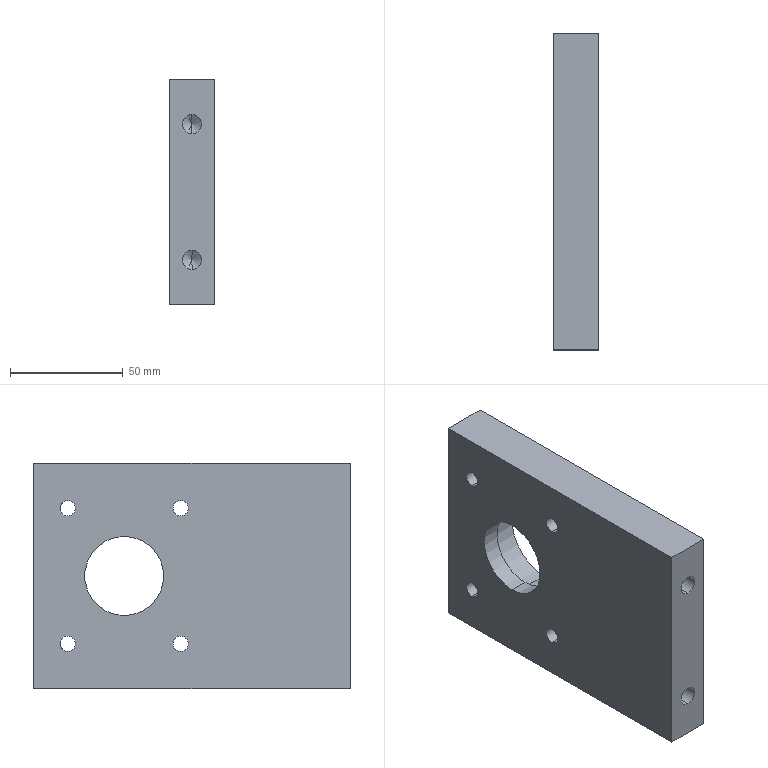Part | SolidWorks | features HoleWzd 3, ICE 2, Extrusion 1 | 1 solid | 31 faces | box 20 x 140 x 100 mm | volume 250976 mm3 | cylinder 20 | plane 7 | cone 4 | commonest cylinder face diameters 6.8 x8 5 x4 8.5 x4 35 x2 40 x2
STEP:
#1=CARTESIAN_POINT('',(10.,57.304,-32.5));
#2=VERTEX_POINT('',#1);
#3=CARTESIAN_POINT('',(10.,57.304,-27.5));
#4=VERTEX_POINT('',#3);
#5=CARTESIAN_POINT('',(10.,57.304,-32.5));
#6=CARTESIAN_POINT('',(9.828,57.304,-32.5));
#7=CARTESIAN_POINT('',(9.657,57.324,-32.482));
#8=CARTESIAN_POINT('',(9.329,57.395,-32.414));
#9=CARTESIAN_POINT('',(9.17,57.445,-32.364));
#10=CARTESIAN_POINT('',(8.728,57.618,-32.176));
#11=CARTESIAN_POINT('',(8.464,57.763,-31.998));
#12=CARTESIAN_POINT('',(8.13,57.966,-31.667));
#13=CARTESIAN_POINT('',(8.027,58.033,-31.544));
#14=CARTESIAN_POINT('',(7.847,58.153,-31.28));
#15=CARTESIAN_POINT('',(7.769,58.207,-31.139));
#16=CARTESIAN_POINT('',(7.638,58.299,-30.836));
#17=CARTESIAN_POINT('',(7.587,58.336,-30.675));
#18=CARTESIAN_POINT('',(7.519,58.386,-30.347));
#19=CARTESIAN_POINT('',(7.5,58.4,-30.176));
#20=CARTESIAN_POINT('',(7.5,58.4,-29.832));
#21=CARTESIAN_POINT('',(7.517,58.387,-29.663));
#22=CARTESIAN_POINT('',(7.585,58.338,-29.331));
#23=CARTESIAN_POINT('',(7.636,58.301,-29.169));
#24=CARTESIAN_POINT('',(7.766,58.209,-28.866));
#25=CARTESIAN_POINT('',(7.845,58.154,-28.722));
#26=CARTESIAN_POINT('',(8.026,58.033,-28.458));
#27=CARTESIAN_POINT('',(8.127,57.968,-28.336));
#28=CARTESIAN_POINT('',(8.464,57.764,-28.003));
#29=CARTESIAN_POINT('',(8.722,57.62,-27.827));
#30=CARTESIAN_POINT('',(9.17,57.445,-27.636));
#31=CARTESIAN_POINT('',(9.326,57.396,-27.587));
#32=CARTESIAN_POINT('',(9.655,57.325,-27.518));
#33=CARTESIAN_POINT('',(9.827,57.304,-27.5));
#34=CARTESIAN_POINT('',(10.,57.304,-27.5));
#35=B_SPLINE_CURVE_WITH_KNOTS('',3,(#5,#6,#7,#8,#9,#10,#11,#12,#13,#14,#15,#16,#17,#18,#19,#20,#21,#22,#23,#24,#25,#26,#27,#28,#29,#30,#31,#32,#33,#34),.UNSPECIFIED.,.F.,.F.,(4,2,2,2,2,2,2,2,2,2,2,2,2,2,4),(0.008147,0.008656,0.009164,0.01018,0.01069,0.0112,0.01171,0.01221,0.01272,0.01323,0.01374,0.01425,0.01526,0.01577,0.01628),.UNSPECIFIED.);
#36=EDGE_CURVE('',#2,#4,#35,.T.);
#37=ORIENTED_EDGE('',*,*,#36,.F.);
#38=CARTESIAN_POINT('',(10.,70.,-32.5));
#39=VERTEX_POINT('',#38);
#40=CARTESIAN_POINT('',(10.,70.,-32.5));
#41=DIRECTION('',(0.,1.,0.));
#42=VECTOR('',#41,1000.);
#43=LINE('',#40,#42);
#44=EDGE_CURVE('',#2,#39,#43,.T.);
#45=ORIENTED_EDGE('',*,*,#44,.T.);
#46=CARTESIAN_POINT('',(10.,70.,-27.5));
#47=VERTEX_POINT('',#46);
#48=CARTESIAN_POINT('',(10.,70.,-30.));
#49=DIRECTION('',(0.,1.,0.));
#50=DIRECTION('',(0.,0.,1.));
#51=AXIS2_PLACEMENT_3D('',#48,#49,#50);
#52=CIRCLE('',#51,2.5);
#53=EDGE_CURVE('',#39,#47,#52,.T.);
#54=ORIENTED_EDGE('',*,*,#53,.T.);
#55=CARTESIAN_POINT('',(10.,70.,-27.5));
#56=DIRECTION('',(0.,1.,0.));
#57=VECTOR('',#56,1000.);
#58=LINE('',#55,#57);
#59=EDGE_CURVE('',#4,#47,#58,.T.);
#60=ORIENTED_EDGE('',*,*,#59,.F.);
#61=EDGE_LOOP('',(#37,#45,#54,#60));
#62=FACE_OUTER_BOUND('',#61,.T.);
#63=CARTESIAN_POINT('',(10.,70.,-30.));
#64=DIRECTION('',(0.,1.,0.));
#65=DIRECTION('',(0.,0.,1.));
#66=AXIS2_PLACEMENT_3D('',#63,#64,#65);
#67=CYLINDRICAL_SURFACE('',#66,2.5);
#68=ADVANCED_FACE('',(#62),#67,.F.);
#69=CARTESIAN_POINT('',(10.,57.304,27.5));
#70=VERTEX_POINT('',#69);
#71=CARTESIAN_POINT('',(10.,57.304,32.5));
#72=VERTEX_POINT('',#71);
#73=CARTESIAN_POINT('',(10.,57.304,27.5));
#74=CARTESIAN_POINT('',(9.828,57.304,27.5));
#75=CARTESIAN_POINT('',(9.657,57.324,27.518));
#76=CARTESIAN_POINT('',(9.329,57.395,27.586));
#77=CARTESIAN_POINT('',(9.17,57.445,27.636));
#78=CARTESIAN_POINT('',(8.728,57.618,27.824));
#79=CARTESIAN_POINT('',(8.464,57.763,28.002));
#80=CARTESIAN_POINT('',(8.13,57.966,28.333));
#81=CARTESIAN_POINT('',(8.027,58.033,28.456));
#82=CARTESIAN_POINT('',(7.847,58.153,28.72));
#83=CARTESIAN_POINT('',(7.769,58.207,28.861));
#84=CARTESIAN_POINT('',(7.638,58.299,29.164));
#85=CARTESIAN_POINT('',(7.587,58.336,29.325));
#86=CARTESIAN_POINT('',(7.519,58.386,29.653));
#87=CARTESIAN_POINT('',(7.5,58.4,29.824));
#88=CARTESIAN_POINT('',(7.5,58.4,30.168));
#89=CARTESIAN_POINT('',(7.517,58.387,30.337));
#90=CARTESIAN_POINT('',(7.585,58.338,30.669));
#91=CARTESIAN_POINT('',(7.636,58.301,30.831));
#92=CARTESIAN_POINT('',(7.766,58.209,31.134));
#93=CARTESIAN_POINT('',(7.845,58.154,31.278));
#94=CARTESIAN_POINT('',(8.026,58.033,31.542));
#95=CARTESIAN_POINT('',(8.127,57.968,31.664));
#96=CARTESIAN_POINT('',(8.464,57.764,31.997));
#97=CARTESIAN_POINT('',(8.722,57.62,32.173));
#98=CARTESIAN_POINT('',(9.17,57.445,32.364));
#99=CARTESIAN_POINT('',(9.326,57.396,32.413));
#100=CARTESIAN_POINT('',(9.655,57.325,32.482));
#101=CARTESIAN_POINT('',(9.827,57.304,32.5));
#102=CARTESIAN_POINT('',(10.,57.304,32.5));
#103=B_SPLINE_CURVE_WITH_KNOTS('',3,(#73,#74,#75,#76,#77,#78,#79,#80,#81,#82,#83,#84,#85,#86,#87,#88,#89,#90,#91,#92,#93,#94,#95,#96,#97,#98,#99,#100,#101,#102),.UNSPECIFIED.,.F.,.F.,(4,2,2,2,2,2,2,2,2,2,2,2,2,2,4),(0.008147,0.008656,0.009164,0.01018,0.01069,0.0112,0.01171,0.01221,0.01272,0.01323,0.01374,0.01425,0.01526,0.01577,0.01628),.UNSPECIFIED.);
#104=EDGE_CURVE('',#70,#72,#103,.T.);
#105=ORIENTED_EDGE('',*,*,#104,.F.);
#106=CARTESIAN_POINT('',(10.,70.,27.5));
#107=VERTEX_POINT('',#106);
#108=CARTESIAN_POINT('',(10.,70.,27.5));
#109=DIRECTION('',(0.,1.,0.));
#110=VECTOR('',#109,1000.);
#111=LINE('',#108,#110);
#112=EDGE_CURVE('',#70,#107,#111,.T.);
#113=ORIENTED_EDGE('',*,*,#112,.T.);
#114=CARTESIAN_POINT('',(10.,70.,32.5));
#115=VERTEX_POINT('',#114);
#116=CARTESIAN_POINT('',(10.,70.,30.));
#117=DIRECTION('',(0.,1.,0.));
#118=DIRECTION('',(0.,0.,1.));
#119=AXIS2_PLACEMENT_3D('',#116,#117,#118);
#120=CIRCLE('',#119,2.5);
#121=EDGE_CURVE('',#107,#115,#120,.T.);
#122=ORIENTED_EDGE('',*,*,#121,.T.);
#123=CARTESIAN_POINT('',(10.,70.,32.5));
#124=DIRECTION('',(0.,1.,0.));
#125=VECTOR('',#124,1000.);
#126=LINE('',#123,#125);
#127=EDGE_CURVE('',#72,#115,#126,.T.);
#128=ORIENTED_EDGE('',*,*,#127,.F.);
#129=EDGE_LOOP('',(#105,#113,#122,#128));
#130=FACE_OUTER_BOUND('',#129,.T.);
#131=CARTESIAN_POINT('',(10.,70.,30.));
#132=DIRECTION('',(0.,1.,0.));
#133=DIRECTION('',(0.,0.,1.));
#134=AXIS2_PLACEMENT_3D('',#131,#132,#133);
#135=CYLINDRICAL_SURFACE('',#134,2.5);
#136=ADVANCED_FACE('',(#130),#135,.F.);
#137=CARTESIAN_POINT('',(20.,55.,-33.4));
#138=VERTEX_POINT('',#137);
#139=CARTESIAN_POINT('',(20.,55.,-26.6));
#140=VERTEX_POINT('',#139);
#141=CARTESIAN_POINT('',(20.,55.,-30.));
#142=DIRECTION('',(-1.,0.,0.));
#143=DIRECTION('',(0.,0.,1.));
#144=AXIS2_PLACEMENT_3D('',#141,#142,#143);
#145=CIRCLE('',#144,3.4);
#146=EDGE_CURVE('',#138,#140,#145,.T.);
#147=ORIENTED_EDGE('',*,*,#146,.F.);
#148=CARTESIAN_POINT('',(0.,55.,-33.4));
#149=VERTEX_POINT('',#148);
#150=CARTESIAN_POINT('',(0.,55.,-33.4));
#151=DIRECTION('',(-1.,0.,0.));
#152=VECTOR('',#151,1000.);
#153=LINE('',#150,#152);
#154=EDGE_CURVE('',#138,#149,#153,.T.);
#155=ORIENTED_EDGE('',*,*,#154,.T.);
#156=CARTESIAN_POINT('',(0.,55.,-26.6));
#157=VERTEX_POINT('',#156);
#158=CARTESIAN_POINT('',(0.,55.,-30.));
#159=DIRECTION('',(-1.,0.,0.));
#160=DIRECTION('',(0.,0.,1.));
#161=AXIS2_PLACEMENT_3D('',#158,#159,#160);
#162=CIRCLE('',#161,3.4);
#163=EDGE_CURVE('',#149,#157,#162,.T.);
#164=ORIENTED_EDGE('',*,*,#163,.T.);
#165=CARTESIAN_POINT('',(0.,55.,-26.6));
#166=DIRECTION('',(-1.,0.,0.));
#167=VECTOR('',#166,1000.);
#168=LINE('',#165,#167);
#169=EDGE_CURVE('',#140,#157,#168,.T.);
#170=ORIENTED_EDGE('',*,*,#169,.F.);
#171=EDGE_LOOP('',(#147,#155,#164,#170));
#172=FACE_OUTER_BOUND('',#171,.T.);
#173=CARTESIAN_POINT('',(0.,55.,-30.));
#174=DIRECTION('',(-1.,0.,0.));
#175=DIRECTION('',(0.,0.,1.));
#176=AXIS2_PLACEMENT_3D('',#173,#174,#175);
#177=CYLINDRICAL_SURFACE('',#176,3.4);
#178=ADVANCED_FACE('',(#172),#177,.F.);
#179=CARTESIAN_POINT('',(20.,55.,26.6));
#180=VERTEX_POINT('',#179);
#181=CARTESIAN_POINT('',(20.,55.,33.4));
#182=VERTEX_POINT('',#181);
#183=CARTESIAN_POINT('',(20.,55.,30.));
#184=DIRECTION('',(-1.,0.,0.));
#185=DIRECTION('',(0.,0.,1.));
#186=AXIS2_PLACEMENT_3D('',#183,#184,#185);
#187=CIRCLE('',#186,3.4);
#188=EDGE_CURVE('',#180,#182,#187,.T.);
#189=ORIENTED_EDGE('',*,*,#188,.F.);
#190=CARTESIAN_POINT('',(0.,55.,26.6));
#191=VERTEX_POINT('',#190);
#192=CARTESIAN_POINT('',(0.,55.,26.6));
#193=DIRECTION('',(-1.,0.,0.));
#194=VECTOR('',#193,1000.);
#195=LINE('',#192,#194);
#196=EDGE_CURVE('',#180,#191,#195,.T.);
#197=ORIENTED_EDGE('',*,*,#196,.T.);
#198=CARTESIAN_POINT('',(0.,55.,33.4));
#199=VERTEX_POINT('',#198);
#200=CARTESIAN_POINT('',(0.,55.,30.));
#201=DIRECTION('',(-1.,0.,0.));
#202=DIRECTION('',(0.,0.,1.));
#203=AXIS2_PLACEMENT_3D('',#200,#201,#202);
#204=CIRCLE('',#203,3.4);
#205=EDGE_CURVE('',#191,#199,#204,.T.);
#206=ORIENTED_EDGE('',*,*,#205,.T.);
#207=CARTESIAN_POINT('',(0.,55.,33.4));
#208=DIRECTION('',(-1.,0.,0.));
#209=VECTOR('',#208,1000.);
#210=LINE('',#207,#209);
#211=EDGE_CURVE('',#182,#199,#210,.T.);
#212=ORIENTED_EDGE('',*,*,#211,.F.);
#213=EDGE_LOOP('',(#189,#197,#206,#212));
#214=FACE_OUTER_BOUND('',#213,.T.);
#215=CARTESIAN_POINT('',(0.,55.,30.));
#216=DIRECTION('',(-1.,0.,0.));
#217=DIRECTION('',(0.,0.,1.));
#218=AXIS2_PLACEMENT_3D('',#215,#216,#217);
#219=CYLINDRICAL_SURFACE('',#218,3.4);
#220=ADVANCED_FACE('',(#214),#219,.F.);
#221=CARTESIAN_POINT('',(20.,5.,-33.4));
#222=VERTEX_POINT('',#221);
#223=CARTESIAN_POINT('',(20.,5.,-26.6));
#224=VERTEX_POINT('',#223);
#225=CARTESIAN_POINT('',(20.,5.,-30.));
#226=DIRECTION('',(-1.,0.,0.));
#227=DIRECTION('',(0.,0.,1.));
#228=AXIS2_PLACEMENT_3D('',#225,#226,#227);
#229=CIRCLE('',#228,3.4);
#230=EDGE_CURVE('',#222,#224,#229,.T.);
#231=ORIENTED_EDGE('',*,*,#230,.F.);
#232=CARTESIAN_POINT('',(0.,5.,-33.4));
#233=VERTEX_POINT('',#232);
#234=CARTESIAN_POINT('',(0.,5.,-33.4));
#235=DIRECTION('',(-1.,0.,0.));
#236=VECTOR('',#235,1000.);
#237=LINE('',#234,#236);
#238=EDGE_CURVE('',#222,#233,#237,.T.);
#239=ORIENTED_EDGE('',*,*,#238,.T.);
#240=CARTESIAN_POINT('',(0.,5.,-26.6));
#241=VERTEX_POINT('',#240);
#242=CARTESIAN_POINT('',(0.,5.,-30.));
#243=DIRECTION('',(-1.,0.,0.));
#244=DIRECTION('',(0.,0.,1.));
#245=AXIS2_PLACEMENT_3D('',#242,#243,#244);
#246=CIRCLE('',#245,3.4);
#247=EDGE_CURVE('',#233,#241,#246,.T.);
#248=ORIENTED_EDGE('',*,*,#247,.T.);
#249=CARTESIAN_POINT('',(0.,5.,-26.6));
#250=DIRECTION('',(-1.,0.,0.));
#251=VECTOR('',#250,1000.);
#252=LINE('',#249,#251);
#253=EDGE_CURVE('',#224,#241,#252,.T.);
#254=ORIENTED_EDGE('',*,*,#253,.F.);
#255=EDGE_LOOP('',(#231,#239,#248,#254));
#256=FACE_OUTER_BOUND('',#255,.T.);
#257=CARTESIAN_POINT('',(0.,5.,-30.));
#258=DIRECTION('',(-1.,0.,0.));
#259=DIRECTION('',(0.,0.,1.));
#260=AXIS2_PLACEMENT_3D('',#257,#258,#259);
#261=CYLINDRICAL_SURFACE('',#260,3.4);
#262=ADVANCED_FACE('',(#256),#261,.F.);
#263=CARTESIAN_POINT('',(20.,5.,26.6));
#264=VERTEX_POINT('',#263);
#265=CARTESIAN_POINT('',(20.,5.,33.4));
#266=VERTEX_POINT('',#265);
#267=CARTESIAN_POINT('',(20.,5.,30.));
#268=DIRECTION('',(-1.,0.,0.));
#269=DIRECTION('',(0.,0.,1.));
#270=AXIS2_PLACEMENT_3D('',#267,#268,#269);
#271=CIRCLE('',#270,3.4);
#272=EDGE_CURVE('',#264,#266,#271,.T.);
#273=ORIENTED_EDGE('',*,*,#272,.F.);
#274=CARTESIAN_POINT('',(0.,5.,26.6));
#275=VERTEX_POINT('',#274);
#276=CARTESIAN_POINT('',(0.,5.,26.6));
#277=DIRECTION('',(-1.,0.,0.));
#278=VECTOR('',#277,1000.);
#279=LINE('',#276,#278);
#280=EDGE_CURVE('',#264,#275,#279,.T.);
#281=ORIENTED_EDGE('',*,*,#280,.T.);
#282=CARTESIAN_POINT('',(0.,5.,33.4));
#283=VERTEX_POINT('',#282);
#284=CARTESIAN_POINT('',(0.,5.,30.));
#285=DIRECTION('',(-1.,0.,0.));
#286=DIRECTION('',(0.,0.,1.));
#287=AXIS2_PLACEMENT_3D('',#284,#285,#286);
#288=CIRCLE('',#287,3.4);
#289=EDGE_CURVE('',#275,#283,#288,.T.);
#290=ORIENTED_EDGE('',*,*,#289,.T.);
#291=CARTESIAN_POINT('',(0.,5.,33.4));
#292=DIRECTION('',(-1.,0.,0.));
#293=VECTOR('',#292,1000.);
#294=LINE('',#291,#293);
#295=EDGE_CURVE('',#266,#283,#294,.T.);
#296=ORIENTED_EDGE('',*,*,#295,.F.);
#297=EDGE_LOOP('',(#273,#281,#290,#296));
#298=FACE_OUTER_BOUND('',#297,.T.);
#299=CARTESIAN_POINT('',(0.,5.,30.));
#300=DIRECTION('',(-1.,0.,0.));
#301=DIRECTION('',(0.,0.,1.));
#302=AXIS2_PLACEMENT_3D('',#299,#300,#301);
#303=CYLINDRICAL_SURFACE('',#302,3.4);
#304=ADVANCED_FACE('',(#298),#303,.F.);
#305=CARTESIAN_POINT('',(0.,30.,17.5));
#306=VERTEX_POINT('',#305);
#307=CARTESIAN_POINT('',(0.,30.,-17.5));
#308=VERTEX_POINT('',#307);
#309=CARTESIAN_POINT('',(0.,30.,0.));
#310=DIRECTION('',(1.,0.,0.));
#311=DIRECTION('',(0.,0.,-1.));
#312=AXIS2_PLACEMENT_3D('',#309,#310,#311);
#313=CIRCLE('',#312,17.5);
#314=EDGE_CURVE('',#306,#308,#313,.T.);
#315=ORIENTED_EDGE('',*,*,#314,.F.);
#316=CARTESIAN_POINT('',(8.,30.,17.5));
#317=VERTEX_POINT('',#316);
#318=CARTESIAN_POINT('',(0.,30.,17.5));
#319=DIRECTION('',(1.,0.,0.));
#320=VECTOR('',#319,1000.);
#321=LINE('',#318,#320);
#322=EDGE_CURVE('',#306,#317,#321,.T.);
#323=ORIENTED_EDGE('',*,*,#322,.T.);
#324=CARTESIAN_POINT('',(8.,30.,-17.5));
#325=VERTEX_POINT('',#324);
#326=CARTESIAN_POINT('',(8.,30.,0.));
#327=DIRECTION('',(1.,0.,0.));
#328=DIRECTION('',(0.,0.,-1.));
#329=AXIS2_PLACEMENT_3D('',#326,#327,#328);
#330=CIRCLE('',#329,17.5);
#331=EDGE_CURVE('',#317,#325,#330,.T.);
#332=ORIENTED_EDGE('',*,*,#331,.T.);
#333=CARTESIAN_POINT('',(0.,30.,-17.5));
#334=DIRECTION('',(1.,0.,0.));
#335=VECTOR('',#334,1000.);
#336=LINE('',#333,#335);
#337=EDGE_CURVE('',#308,#325,#336,.T.);
#338=ORIENTED_EDGE('',*,*,#337,.F.);
#339=EDGE_LOOP('',(#315,#323,#332,#338));
#340=FACE_OUTER_BOUND('',#339,.T.);
#341=CARTESIAN_POINT('',(0.,30.,0.));
#342=DIRECTION('',(1.,0.,0.));
#343=DIRECTION('',(0.,0.,-1.));
#344=AXIS2_PLACEMENT_3D('',#341,#342,#343);
#345=CYLINDRICAL_SURFACE('',#344,17.5);
#346=ADVANCED_FACE('',(#340),#345,.F.);
#347=CARTESIAN_POINT('',(8.,30.,20.));
#348=VERTEX_POINT('',#347);
#349=CARTESIAN_POINT('',(8.,30.,-20.));
#350=VERTEX_POINT('',#349);
#351=CARTESIAN_POINT('',(8.,30.,0.));
#352=DIRECTION('',(1.,0.,0.));
#353=DIRECTION('',(0.,0.,-1.));
#354=AXIS2_PLACEMENT_3D('',#351,#352,#353);
#355=CIRCLE('',#354,20.);
#356=EDGE_CURVE('',#348,#350,#355,.T.);
#357=ORIENTED_EDGE('',*,*,#356,.F.);
#358=CARTESIAN_POINT('',(20.,30.,20.));
#359=VERTEX_POINT('',#358);
#360=CARTESIAN_POINT('',(8.,30.,20.));
#361=DIRECTION('',(1.,0.,0.));
#362=VECTOR('',#361,1000.);
#363=LINE('',#360,#362);
#364=EDGE_CURVE('',#348,#359,#363,.T.);
#365=ORIENTED_EDGE('',*,*,#364,.T.);
#366=CARTESIAN_POINT('',(20.,30.,-20.));
#367=VERTEX_POINT('',#366);
#368=CARTESIAN_POINT('',(20.,30.,0.));
#369=DIRECTION('',(1.,0.,0.));
#370=DIRECTION('',(0.,0.,-1.));
#371=AXIS2_PLACEMENT_3D('',#368,#369,#370);
#372=CIRCLE('',#371,20.);
#373=EDGE_CURVE('',#359,#367,#372,.T.);
#374=ORIENTED_EDGE('',*,*,#373,.T.);
#375=CARTESIAN_POINT('',(8.,30.,-20.));
#376=DIRECTION('',(1.,0.,0.));
#377=VECTOR('',#376,1000.);
#378=LINE('',#375,#377);
#379=EDGE_CURVE('',#350,#367,#378,.T.);
#380=ORIENTED_EDGE('',*,*,#379,.F.);
#381=EDGE_LOOP('',(#357,#365,#374,#380));
#382=FACE_OUTER_BOUND('',#381,.T.);
#383=CARTESIAN_POINT('',(8.,30.,0.));
#384=DIRECTION('',(1.,0.,0.));
#385=DIRECTION('',(0.,0.,-1.));
#386=AXIS2_PLACEMENT_3D('',#383,#384,#385);
#387=CYLINDRICAL_SURFACE('',#386,20.);
#388=ADVANCED_FACE('',(#382),#387,.F.);
#389=CARTESIAN_POINT('',(10.,-45.5,-25.75));
#390=VERTEX_POINT('',#389);
#391=CARTESIAN_POINT('',(10.,-45.5,-34.25));
#392=VERTEX_POINT('',#391);
#393=CARTESIAN_POINT('',(10.,-45.5,-30.));
#394=DIRECTION('',(0.,-1.,0.));
#395=DIRECTION('',(0.,0.,-1.));
#396=AXIS2_PLACEMENT_3D('',#393,#394,#395);
#397=CIRCLE('',#396,4.25);
#398=EDGE_CURVE('',#390,#392,#397,.T.);
#399=ORIENTED_EDGE('',*,*,#398,.F.);
#400=CARTESIAN_POINT('',(10.,-70.,-25.75));
#401=VERTEX_POINT('',#400);
#402=CARTESIAN_POINT('',(10.,-70.,-25.75));
#403=DIRECTION('',(0.,-1.,0.));
#404=VECTOR('',#403,1000.);
#405=LINE('',#402,#404);
#406=EDGE_CURVE('',#390,#401,#405,.T.);
#407=ORIENTED_EDGE('',*,*,#406,.T.);
#408=CARTESIAN_POINT('',(10.,-70.,-34.25));
#409=VERTEX_POINT('',#408);
#410=CARTESIAN_POINT('',(10.,-70.,-30.));
#411=DIRECTION('',(0.,-1.,0.));
#412=DIRECTION('',(0.,0.,-1.));
#413=AXIS2_PLACEMENT_3D('',#410,#411,#412);
#414=CIRCLE('',#413,4.25);
#415=EDGE_CURVE('',#401,#409,#414,.T.);
#416=ORIENTED_EDGE('',*,*,#415,.T.);
#417=CARTESIAN_POINT('',(10.,-70.,-34.25));
#418=DIRECTION('',(0.,-1.,0.));
#419=VECTOR('',#418,1000.);
#420=LINE('',#417,#419);
#421=EDGE_CURVE('',#392,#409,#420,.T.);
#422=ORIENTED_EDGE('',*,*,#421,.F.);
#423=EDGE_LOOP('',(#399,#407,#416,#422));
#424=FACE_OUTER_BOUND('',#423,.T.);
#425=CARTESIAN_POINT('',(10.,-70.,-30.));
#426=DIRECTION('',(0.,-1.,0.));
#427=DIRECTION('',(0.,0.,-1.));
#428=AXIS2_PLACEMENT_3D('',#425,#426,#427);
#429=CYLINDRICAL_SURFACE('',#428,4.25);
#430=ADVANCED_FACE('',(#424),#429,.F.);
#431=CARTESIAN_POINT('',(10.,-42.946,-30.));
#432=VERTEX_POINT('',#431);
#433=CARTESIAN_POINT('',(10.,-45.5,-34.25));
#434=DIRECTION('',(0.,-0.515,-0.8572));
#435=VECTOR('',#434,1000.);
#436=LINE('',#433,#435);
#437=EDGE_CURVE('',#432,#392,#436,.T.);
#438=ORIENTED_EDGE('',*,*,#437,.F.);
#439=CARTESIAN_POINT('',(10.,-45.5,-25.75));
#440=DIRECTION('',(0.,-0.515,0.8572));
#441=VECTOR('',#440,1000.);
#442=LINE('',#439,#441);
#443=EDGE_CURVE('',#432,#390,#442,.T.);
#444=ORIENTED_EDGE('',*,*,#443,.T.);
#445=ORIENTED_EDGE('',*,*,#398,.T.);
#446=EDGE_LOOP('',(#438,#444,#445));
#447=FACE_OUTER_BOUND('',#446,.T.);
#448=CARTESIAN_POINT('',(10.,-45.5,-30.));
#449=DIRECTION('',(0.,-1.,0.));
#450=DIRECTION('',(0.,0.,-1.));
#451=AXIS2_PLACEMENT_3D('',#448,#449,#450);
#452=CONICAL_SURFACE('',#451,4.25,1.03);
#453=ADVANCED_FACE('',(#447),#452,.F.);
#454=CARTESIAN_POINT('',(10.,-45.5,34.25));
#455=VERTEX_POINT('',#454);
#456=CARTESIAN_POINT('',(10.,-45.5,25.75));
#457=VERTEX_POINT('',#456);
#458=CARTESIAN_POINT('',(10.,-45.5,30.));
#459=DIRECTION('',(0.,-1.,0.));
#460=DIRECTION('',(0.,0.,-1.));
#461=AXIS2_PLACEMENT_3D('',#458,#459,#460);
#462=CIRCLE('',#461,4.25);
#463=EDGE_CURVE('',#455,#457,#462,.T.);
#464=ORIENTED_EDGE('',*,*,#463,.F.);
#465=CARTESIAN_POINT('',(10.,-70.,34.25));
#466=VERTEX_POINT('',#465);
#467=CARTESIAN_POINT('',(10.,-70.,34.25));
#468=DIRECTION('',(0.,-1.,0.));
#469=VECTOR('',#468,1000.);
#470=LINE('',#467,#469);
#471=EDGE_CURVE('',#455,#466,#470,.T.);
#472=ORIENTED_EDGE('',*,*,#471,.T.);
#473=CARTESIAN_POINT('',(10.,-70.,25.75));
#474=VERTEX_POINT('',#473);
#475=CARTESIAN_POINT('',(10.,-70.,30.));
#476=DIRECTION('',(0.,-1.,0.));
#477=DIRECTION('',(0.,0.,-1.));
#478=AXIS2_PLACEMENT_3D('',#475,#476,#477);
#479=CIRCLE('',#478,4.25);
#480=EDGE_CURVE('',#466,#474,#479,.T.);
#481=ORIENTED_EDGE('',*,*,#480,.T.);
#482=CARTESIAN_POINT('',(10.,-70.,25.75));
#483=DIRECTION('',(0.,-1.,0.));
#484=VECTOR('',#483,1000.);
#485=LINE('',#482,#484);
#486=EDGE_CURVE('',#457,#474,#485,.T.);
#487=ORIENTED_EDGE('',*,*,#486,.F.);
#488=EDGE_LOOP('',(#464,#472,#481,#487));
#489=FACE_OUTER_BOUND('',#488,.T.);
#490=CARTESIAN_POINT('',(10.,-70.,30.));
#491=DIRECTION('',(0.,-1.,0.));
#492=DIRECTION('',(0.,0.,-1.));
#493=AXIS2_PLACEMENT_3D('',#490,#491,#492);
#494=CYLINDRICAL_SURFACE('',#493,4.25);
#495=ADVANCED_FACE('',(#489),#494,.F.);
#496=CARTESIAN_POINT('',(10.,-42.946,30.));
#497=VERTEX_POINT('',#496);
#498=CARTESIAN_POINT('',(10.,-45.5,25.75));
#499=DIRECTION('',(0.,-0.515,-0.8572));
#500=VECTOR('',#499,1000.);
#501=LINE('',#498,#500);
#502=EDGE_CURVE('',#497,#457,#501,.T.);
#503=ORIENTED_EDGE('',*,*,#502,.F.);
#504=CARTESIAN_POINT('',(10.,-45.5,34.25));
#505=DIRECTION('',(0.,-0.515,0.8572));
#506=VECTOR('',#505,1000.);
#507=LINE('',#504,#506);
#508=EDGE_CURVE('',#497,#455,#507,.T.);
#509=ORIENTED_EDGE('',*,*,#508,.T.);
#510=ORIENTED_EDGE('',*,*,#463,.T.);
#511=EDGE_LOOP('',(#503,#509,#510));
#512=FACE_OUTER_BOUND('',#511,.T.);
#513=CARTESIAN_POINT('',(10.,-45.5,30.));
#514=DIRECTION('',(0.,-1.,0.));
#515=DIRECTION('',(0.,0.,-1.));
#516=AXIS2_PLACEMENT_3D('',#513,#514,#515);
#517=CONICAL_SURFACE('',#516,4.25,1.03);
#518=ADVANCED_FACE('',(#512),#517,.F.);
#519=CARTESIAN_POINT('',(0.,55.,-30.));
#520=DIRECTION('',(-1.,0.,0.));
#521=DIRECTION('',(0.,0.,1.));
#522=AXIS2_PLACEMENT_3D('',#519,#520,#521);
#523=CIRCLE('',#522,3.4);
#524=EDGE_CURVE('',#157,#149,#523,.T.);
#525=ORIENTED_EDGE('',*,*,#524,.F.);
#526=ORIENTED_EDGE('',*,*,#163,.F.);
#527=EDGE_LOOP('',(#525,#526));
#528=FACE_BOUND('',#527,.T.);
#529=CARTESIAN_POINT('',(0.,5.,-30.));
#530=DIRECTION('',(-1.,0.,0.));
#531=DIRECTION('',(0.,0.,1.));
#532=AXIS2_PLACEMENT_3D('',#529,#530,#531);
#533=CIRCLE('',#532,3.4);
#534=EDGE_CURVE('',#241,#233,#533,.T.);
#535=ORIENTED_EDGE('',*,*,#534,.F.);
#536=ORIENTED_EDGE('',*,*,#247,.F.);
#537=EDGE_LOOP('',(#535,#536));
#538=FACE_BOUND('',#537,.T.);
#539=CARTESIAN_POINT('',(0.,5.,30.));
#540=DIRECTION('',(-1.,0.,0.));
#541=DIRECTION('',(0.,0.,1.));
#542=AXIS2_PLACEMENT_3D('',#539,#540,#541);
#543=CIRCLE('',#542,3.4);
#544=EDGE_CURVE('',#283,#275,#543,.T.);
#545=ORIENTED_EDGE('',*,*,#544,.F.);
#546=ORIENTED_EDGE('',*,*,#289,.F.);
#547=EDGE_LOOP('',(#545,#546));
#548=FACE_BOUND('',#547,.T.);
#549=CARTESIAN_POINT('',(0.,30.,0.));
#550=DIRECTION('',(1.,0.,0.));
#551=DIRECTION('',(0.,0.,-1.));
#552=AXIS2_PLACEMENT_3D('',#549,#550,#551);
#553=CIRCLE('',#552,17.5);
#554=EDGE_CURVE('',#308,#306,#553,.T.);
#555=ORIENTED_EDGE('',*,*,#554,.T.);
#556=ORIENTED_EDGE('',*,*,#314,.T.);
#557=EDGE_LOOP('',(#555,#556));
#558=FACE_BOUND('',#557,.T.);
#559=CARTESIAN_POINT('',(0.,-70.,-50.));
#560=VERTEX_POINT('',#559);
#561=CARTESIAN_POINT('',(0.,70.,-50.));
#562=VERTEX_POINT('',#561);
#563=CARTESIAN_POINT('',(0.,70.,-50.));
#564=DIRECTION('',(0.,1.,0.));
#565=VECTOR('',#564,1000.);
#566=LINE('',#563,#565);
#567=EDGE_CURVE('',#560,#562,#566,.T.);
#568=ORIENTED_EDGE('',*,*,#567,.F.);
#569=CARTESIAN_POINT('',(0.,-70.,50.));
#570=VERTEX_POINT('',#569);
#571=CARTESIAN_POINT('',(0.,-70.,50.));
#572=DIRECTION('',(0.,0.,-1.));
#573=VECTOR('',#572,1000.);
#574=LINE('',#571,#573);
#575=EDGE_CURVE('',#570,#560,#574,.T.);
#576=ORIENTED_EDGE('',*,*,#575,.F.);
#577=CARTESIAN_POINT('',(0.,70.,50.));
#578=VERTEX_POINT('',#577);
#579=CARTESIAN_POINT('',(0.,70.,50.));
#580=DIRECTION('',(0.,-1.,0.));
#581=VECTOR('',#580,1000.);
#582=LINE('',#579,#581);
#583=EDGE_CURVE('',#578,#570,#582,.T.);
#584=ORIENTED_EDGE('',*,*,#583,.F.);
#585=CARTESIAN_POINT('',(0.,70.,50.));
#586=DIRECTION('',(0.,0.,1.));
#587=VECTOR('',#586,1000.);
#588=LINE('',#585,#587);
#589=EDGE_CURVE('',#562,#578,#588,.T.);
#590=ORIENTED_EDGE('',*,*,#589,.F.);
#591=EDGE_LOOP('',(#568,#576,#584,#590));
#592=FACE_OUTER_BOUND('',#591,.T.);
#593=CARTESIAN_POINT('',(0.,55.,30.));
#594=DIRECTION('',(-1.,0.,0.));
#595=DIRECTION('',(0.,0.,1.));
#596=AXIS2_PLACEMENT_3D('',#593,#594,#595);
#597=CIRCLE('',#596,3.4);
#598=EDGE_CURVE('',#199,#191,#597,.T.);
#599=ORIENTED_EDGE('',*,*,#598,.F.);
#600=ORIENTED_EDGE('',*,*,#205,.F.);
#601=EDGE_LOOP('',(#599,#600));
#602=FACE_BOUND('',#601,.T.);
#603=CARTESIAN_POINT('',(0.,0.,0.));
#604=DIRECTION('',(1.,0.,0.));
#605=DIRECTION('',(0.,0.,-1.));
#606=AXIS2_PLACEMENT_3D('',#603,#604,#605);
#607=PLANE('',#606);
#608=ADVANCED_FACE('',(#528,#538,#548,#558,#592,#602),#607,.F.);
#609=ORIENTED_EDGE('',*,*,#567,.T.);
#610=CARTESIAN_POINT('',(20.,70.,-50.));
#611=VERTEX_POINT('',#610);
#612=CARTESIAN_POINT('',(20.,70.,-50.));
#613=DIRECTION('',(-1.,0.,0.));
#614=VECTOR('',#613,1000.);
#615=LINE('',#612,#614);
#616=EDGE_CURVE('',#611,#562,#615,.T.);
#617=ORIENTED_EDGE('',*,*,#616,.F.);
#618=CARTESIAN_POINT('',(20.,-70.,-50.));
#619=VERTEX_POINT('',#618);
#620=CARTESIAN_POINT('',(20.,70.,-50.));
#621=DIRECTION('',(0.,1.,0.));
#622=VECTOR('',#621,1000.);
#623=LINE('',#620,#622);
#624=EDGE_CURVE('',#619,#611,#623,.T.);
#625=ORIENTED_EDGE('',*,*,#624,.F.);
#626=CARTESIAN_POINT('',(20.,-70.,-50.));
#627=DIRECTION('',(-1.,0.,0.));
#628=VECTOR('',#627,1000.);
#629=LINE('',#626,#628);
#630=EDGE_CURVE('',#619,#560,#629,.T.);
#631=ORIENTED_EDGE('',*,*,#630,.T.);
#632=EDGE_LOOP('',(#609,#617,#625,#631));
#633=FACE_OUTER_BOUND('',#632,.T.);
#634=CARTESIAN_POINT('',(20.,70.,-50.));
#635=DIRECTION('',(0.,0.,1.));
#636=DIRECTION('',(0.,-1.,0.));
#637=AXIS2_PLACEMENT_3D('',#634,#635,#636);
#638=PLANE('',#637);
#639=ADVANCED_FACE('',(#633),#638,.F.);
#640=CARTESIAN_POINT('',(10.,70.,-30.));
#641=DIRECTION('',(0.,1.,0.));
#642=DIRECTION('',(0.,0.,1.));
#643=AXIS2_PLACEMENT_3D('',#640,#641,#642);
#644=CIRCLE('',#643,2.5);
#645=EDGE_CURVE('',#47,#39,#644,.T.);
#646=ORIENTED_EDGE('',*,*,#645,.F.);
#647=ORIENTED_EDGE('',*,*,#53,.F.);
#648=EDGE_LOOP('',(#646,#647));
#649=FACE_BOUND('',#648,.T.);
#650=CARTESIAN_POINT('',(10.,70.,30.));
#651=DIRECTION('',(0.,1.,0.));
#652=DIRECTION('',(0.,0.,1.));
#653=AXIS2_PLACEMENT_3D('',#650,#651,#652);
#654=CIRCLE('',#653,2.5);
#655=EDGE_CURVE('',#115,#107,#654,.T.);
#656=ORIENTED_EDGE('',*,*,#655,.F.);
#657=ORIENTED_EDGE('',*,*,#121,.F.);
#658=EDGE_LOOP('',(#656,#657));
#659=FACE_BOUND('',#658,.T.);
#660=ORIENTED_EDGE('',*,*,#589,.T.);
#661=CARTESIAN_POINT('',(20.,70.,50.));
#662=VERTEX_POINT('',#661);
#663=CARTESIAN_POINT('',(20.,70.,50.));
#664=DIRECTION('',(-1.,0.,0.));
#665=VECTOR('',#664,1000.);
#666=LINE('',#663,#665);
#667=EDGE_CURVE('',#662,#578,#666,.T.);
#668=ORIENTED_EDGE('',*,*,#667,.F.);
#669=CARTESIAN_POINT('',(20.,70.,50.));
#670=DIRECTION('',(0.,0.,1.));
#671=VECTOR('',#670,1000.);
#672=LINE('',#669,#671);
#673=EDGE_CURVE('',#611,#662,#672,.T.);
#674=ORIENTED_EDGE('',*,*,#673,.F.);
#675=ORIENTED_EDGE('',*,*,#616,.T.);
#676=EDGE_LOOP('',(#660,#668,#674,#675));
#677=FACE_OUTER_BOUND('',#676,.T.);
#678=CARTESIAN_POINT('',(20.,70.,50.));
#679=DIRECTION('',(0.,-1.,0.));
#680=DIRECTION('',(0.,0.,-1.));
#681=AXIS2_PLACEMENT_3D('',#678,#679,#680);
#682=PLANE('',#681);
#683=ADVANCED_FACE('',(#649,#659,#677),#682,.F.);
#684=ORIENTED_EDGE('',*,*,#583,.T.);
#685=CARTESIAN_POINT('',(20.,-70.,50.));
#686=VERTEX_POINT('',#685);
#687=CARTESIAN_POINT('',(20.,-70.,50.));
#688=DIRECTION('',(-1.,0.,0.));
#689=VECTOR('',#688,1000.);
#690=LINE('',#687,#689);
#691=EDGE_CURVE('',#686,#570,#690,.T.);
#692=ORIENTED_EDGE('',*,*,#691,.F.);
#693=CARTESIAN_POINT('',(20.,70.,50.));
#694=DIRECTION('',(0.,-1.,0.));
#695=VECTOR('',#694,1000.);
#696=LINE('',#693,#695);
#697=EDGE_CURVE('',#662,#686,#696,.T.);
#698=ORIENTED_EDGE('',*,*,#697,.F.);
#699=ORIENTED_EDGE('',*,*,#667,.T.);
#700=EDGE_LOOP('',(#684,#692,#698,#699));
#701=FACE_OUTER_BOUND('',#700,.T.);
#702=CARTESIAN_POINT('',(20.,70.,50.));
#703=DIRECTION('',(0.,0.,-1.));
#704=DIRECTION('',(0.,1.,0.));
#705=AXIS2_PLACEMENT_3D('',#702,#703,#704);
#706=PLANE('',#705);
#707=ADVANCED_FACE('',(#701),#706,.F.);
#708=CARTESIAN_POINT('',(10.,-70.,-30.));
#709=DIRECTION('',(0.,-1.,0.));
#710=DIRECTION('',(0.,0.,-1.));
#711=AXIS2_PLACEMENT_3D('',#708,#709,#710);
#712=CIRCLE('',#711,4.25);
#713=EDGE_CURVE('',#409,#401,#712,.T.);
#714=ORIENTED_EDGE('',*,*,#713,.F.);
#715=ORIENTED_EDGE('',*,*,#415,.F.);
#716=EDGE_LOOP('',(#714,#715));
#717=FACE_BOUND('',#716,.T.);
#718=CARTESIAN_POINT('',(10.,-70.,30.));
#719=DIRECTION('',(0.,-1.,0.));
#720=DIRECTION('',(0.,0.,-1.));
#721=AXIS2_PLACEMENT_3D('',#718,#719,#720);
#722=CIRCLE('',#721,4.25);
#723=EDGE_CURVE('',#474,#466,#722,.T.);
#724=ORIENTED_EDGE('',*,*,#723,.F.);
#725=ORIENTED_EDGE('',*,*,#480,.F.);
#726=EDGE_LOOP('',(#724,#725));
#727=FACE_BOUND('',#726,.T.);
#728=ORIENTED_EDGE('',*,*,#575,.T.);
#729=ORIENTED_EDGE('',*,*,#630,.F.);
#730=CARTESIAN_POINT('',(20.,-70.,50.));
#731=DIRECTION('',(0.,0.,-1.));
#732=VECTOR('',#731,1000.);
#733=LINE('',#730,#732);
#734=EDGE_CURVE('',#686,#619,#733,.T.);
#735=ORIENTED_EDGE('',*,*,#734,.F.);
#736=ORIENTED_EDGE('',*,*,#691,.T.);
#737=EDGE_LOOP('',(#728,#729,#735,#736));
#738=FACE_OUTER_BOUND('',#737,.T.);
#739=CARTESIAN_POINT('',(20.,-70.,50.));
#740=DIRECTION('',(0.,1.,0.));
#741=DIRECTION('',(0.,0.,1.));
#742=AXIS2_PLACEMENT_3D('',#739,#740,#741);
#743=PLANE('',#742);
#744=ADVANCED_FACE('',(#717,#727,#738),#743,.F.);
#745=CARTESIAN_POINT('',(20.,55.,-30.));
#746=DIRECTION('',(-1.,0.,0.));
#747=DIRECTION('',(0.,0.,1.));
#748=AXIS2_PLACEMENT_3D('',#745,#746,#747);
#749=CIRCLE('',#748,3.4);
#750=EDGE_CURVE('',#140,#138,#749,.T.);
#751=ORIENTED_EDGE('',*,*,#750,.T.);
#752=ORIENTED_EDGE('',*,*,#146,.T.);
#753=EDGE_LOOP('',(#751,#752));
#754=FACE_BOUND('',#753,.T.);
#755=CARTESIAN_POINT('',(20.,55.,30.));
#756=DIRECTION('',(-1.,0.,0.));
#757=DIRECTION('',(0.,0.,1.));
#758=AXIS2_PLACEMENT_3D('',#755,#756,#757);
#759=CIRCLE('',#758,3.4);
#760=EDGE_CURVE('',#182,#180,#759,.T.);
#761=ORIENTED_EDGE('',*,*,#760,.T.);
#762=ORIENTED_EDGE('',*,*,#188,.T.);
#763=EDGE_LOOP('',(#761,#762));
#764=FACE_BOUND('',#763,.T.);
#765=CARTESIAN_POINT('',(20.,5.,-30.));
#766=DIRECTION('',(-1.,0.,0.));
#767=DIRECTION('',(0.,0.,1.));
#768=AXIS2_PLACEMENT_3D('',#765,#766,#767);
#769=CIRCLE('',#768,3.4);
#770=EDGE_CURVE('',#224,#222,#769,.T.);
#771=ORIENTED_EDGE('',*,*,#770,.T.);
#772=ORIENTED_EDGE('',*,*,#230,.T.);
#773=EDGE_LOOP('',(#771,#772));
#774=FACE_BOUND('',#773,.T.);
#775=CARTESIAN_POINT('',(20.,5.,30.));
#776=DIRECTION('',(-1.,0.,0.));
#777=DIRECTION('',(0.,0.,1.));
#778=AXIS2_PLACEMENT_3D('',#775,#776,#777);
#779=CIRCLE('',#778,3.4);
#780=EDGE_CURVE('',#266,#264,#779,.T.);
#781=ORIENTED_EDGE('',*,*,#780,.T.);
#782=ORIENTED_EDGE('',*,*,#272,.T.);
#783=EDGE_LOOP('',(#781,#782));
#784=FACE_BOUND('',#783,.T.);
#785=CARTESIAN_POINT('',(20.,30.,0.));
#786=DIRECTION('',(1.,0.,0.));
#787=DIRECTION('',(0.,0.,-1.));
#788=AXIS2_PLACEMENT_3D('',#785,#786,#787);
#789=CIRCLE('',#788,20.);
#790=EDGE_CURVE('',#367,#359,#789,.T.);
#791=ORIENTED_EDGE('',*,*,#790,.F.);
#792=ORIENTED_EDGE('',*,*,#373,.F.);
#793=EDGE_LOOP('',(#791,#792));
#794=FACE_BOUND('',#793,.T.);
#795=ORIENTED_EDGE('',*,*,#624,.T.);
#796=ORIENTED_EDGE('',*,*,#673,.T.);
#797=ORIENTED_EDGE('',*,*,#697,.T.);
#798=ORIENTED_EDGE('',*,*,#734,.T.);
#799=EDGE_LOOP('',(#795,#796,#797,#798));
#800=FACE_OUTER_BOUND('',#799,.T.);
#801=CARTESIAN_POINT('',(20.,0.,0.));
#802=DIRECTION('',(1.,0.,0.));
#803=DIRECTION('',(0.,0.,-1.));
#804=AXIS2_PLACEMENT_3D('',#801,#802,#803);
#805=PLANE('',#804);
#806=ADVANCED_FACE('',(#754,#764,#774,#784,#794,#800),#805,.T.);
#807=ORIENTED_EDGE('',*,*,#508,.F.);
#808=ORIENTED_EDGE('',*,*,#502,.T.);
#809=CARTESIAN_POINT('',(10.,-45.5,30.));
#810=DIRECTION('',(0.,-1.,0.));
#811=DIRECTION('',(0.,0.,-1.));
#812=AXIS2_PLACEMENT_3D('',#809,#810,#811);
#813=CIRCLE('',#812,4.25);
#814=EDGE_CURVE('',#457,#455,#813,.T.);
#815=ORIENTED_EDGE('',*,*,#814,.T.);
#816=EDGE_LOOP('',(#807,#808,#815));
#817=FACE_OUTER_BOUND('',#816,.T.);
#818=CARTESIAN_POINT('',(10.,-45.5,30.));
#819=DIRECTION('',(0.,-1.,0.));
#820=DIRECTION('',(0.,0.,-1.));
#821=AXIS2_PLACEMENT_3D('',#818,#819,#820);
#822=CONICAL_SURFACE('',#821,4.25,1.03);
#823=ADVANCED_FACE('',(#817),#822,.F.);
#824=ORIENTED_EDGE('',*,*,#471,.F.);
#825=ORIENTED_EDGE('',*,*,#814,.F.);
#826=ORIENTED_EDGE('',*,*,#486,.T.);
#827=ORIENTED_EDGE('',*,*,#723,.T.);
#828=EDGE_LOOP('',(#824,#825,#826,#827));
#829=FACE_OUTER_BOUND('',#828,.T.);
#830=CARTESIAN_POINT('',(10.,-70.,30.));
#831=DIRECTION('',(0.,-1.,0.));
#832=DIRECTION('',(0.,0.,-1.));
#833=AXIS2_PLACEMENT_3D('',#830,#831,#832);
#834=CYLINDRICAL_SURFACE('',#833,4.25);
#835=ADVANCED_FACE('',(#829),#834,.F.);
#836=ORIENTED_EDGE('',*,*,#443,.F.);
#837=ORIENTED_EDGE('',*,*,#437,.T.);
#838=CARTESIAN_POINT('',(10.,-45.5,-30.));
#839=DIRECTION('',(0.,-1.,0.));
#840=DIRECTION('',(0.,0.,-1.));
#841=AXIS2_PLACEMENT_3D('',#838,#839,#840);
#842=CIRCLE('',#841,4.25);
#843=EDGE_CURVE('',#392,#390,#842,.T.);
#844=ORIENTED_EDGE('',*,*,#843,.T.);
#845=EDGE_LOOP('',(#836,#837,#844));
#846=FACE_OUTER_BOUND('',#845,.T.);
#847=CARTESIAN_POINT('',(10.,-45.5,-30.));
#848=DIRECTION('',(0.,-1.,0.));
#849=DIRECTION('',(0.,0.,-1.));
#850=AXIS2_PLACEMENT_3D('',#847,#848,#849);
#851=CONICAL_SURFACE('',#850,4.25,1.03);
#852=ADVANCED_FACE('',(#846),#851,.F.);
#853=ORIENTED_EDGE('',*,*,#406,.F.);
#854=ORIENTED_EDGE('',*,*,#843,.F.);
#855=ORIENTED_EDGE('',*,*,#421,.T.);
#856=ORIENTED_EDGE('',*,*,#713,.T.);
#857=EDGE_LOOP('',(#853,#854,#855,#856));
#858=FACE_OUTER_BOUND('',#857,.T.);
#859=CARTESIAN_POINT('',(10.,-70.,-30.));
#860=DIRECTION('',(0.,-1.,0.));
#861=DIRECTION('',(0.,0.,-1.));
#862=AXIS2_PLACEMENT_3D('',#859,#860,#861);
#863=CYLINDRICAL_SURFACE('',#862,4.25);
#864=ADVANCED_FACE('',(#858),#863,.F.);
#865=ORIENTED_EDGE('',*,*,#364,.F.);
#866=CARTESIAN_POINT('',(8.,30.,0.));
#867=DIRECTION('',(1.,0.,0.));
#868=DIRECTION('',(0.,0.,-1.));
#869=AXIS2_PLACEMENT_3D('',#866,#867,#868);
#870=CIRCLE('',#869,20.);
#871=EDGE_CURVE('',#350,#348,#870,.T.);
#872=ORIENTED_EDGE('',*,*,#871,.F.);
#873=ORIENTED_EDGE('',*,*,#379,.T.);
#874=ORIENTED_EDGE('',*,*,#790,.T.);
#875=EDGE_LOOP('',(#865,#872,#873,#874));
#876=FACE_OUTER_BOUND('',#875,.T.);
#877=CARTESIAN_POINT('',(8.,30.,0.));
#878=DIRECTION('',(1.,0.,0.));
#879=DIRECTION('',(0.,0.,-1.));
#880=AXIS2_PLACEMENT_3D('',#877,#878,#879);
#881=CYLINDRICAL_SURFACE('',#880,20.);
#882=ADVANCED_FACE('',(#876),#881,.F.);
#883=CARTESIAN_POINT('',(8.,30.,0.));
#884=DIRECTION('',(1.,0.,0.));
#885=DIRECTION('',(0.,0.,-1.));
#886=AXIS2_PLACEMENT_3D('',#883,#884,#885);
#887=CIRCLE('',#886,17.5);
#888=EDGE_CURVE('',#325,#317,#887,.T.);
#889=ORIENTED_EDGE('',*,*,#888,.F.);
#890=ORIENTED_EDGE('',*,*,#331,.F.);
#891=EDGE_LOOP('',(#889,#890));
#892=FACE_BOUND('',#891,.T.);
#893=ORIENTED_EDGE('',*,*,#871,.T.);
#894=ORIENTED_EDGE('',*,*,#356,.T.);
#895=EDGE_LOOP('',(#893,#894));
#896=FACE_OUTER_BOUND('',#895,.T.);
#897=CARTESIAN_POINT('',(8.,30.,0.));
#898=DIRECTION('',(1.,0.,0.));
#899=DIRECTION('',(0.,0.,-1.));
#900=AXIS2_PLACEMENT_3D('',#897,#898,#899);
#901=PLANE('',#900);
#902=ADVANCED_FACE('',(#892,#896),#901,.T.);
#903=ORIENTED_EDGE('',*,*,#322,.F.);
#904=ORIENTED_EDGE('',*,*,#554,.F.);
#905=ORIENTED_EDGE('',*,*,#337,.T.);
#906=ORIENTED_EDGE('',*,*,#888,.T.);
#907=EDGE_LOOP('',(#903,#904,#905,#906));
#908=FACE_OUTER_BOUND('',#907,.T.);
#909=CARTESIAN_POINT('',(0.,30.,0.));
#910=DIRECTION('',(1.,0.,0.));
#911=DIRECTION('',(0.,0.,-1.));
#912=AXIS2_PLACEMENT_3D('',#909,#910,#911);
#913=CYLINDRICAL_SURFACE('',#912,17.5);
#914=ADVANCED_FACE('',(#908),#913,.F.);
#915=ORIENTED_EDGE('',*,*,#280,.F.);
#916=ORIENTED_EDGE('',*,*,#780,.F.);
#917=ORIENTED_EDGE('',*,*,#295,.T.);
#918=ORIENTED_EDGE('',*,*,#544,.T.);
#919=EDGE_LOOP('',(#915,#916,#917,#918));
#920=FACE_OUTER_BOUND('',#919,.T.);
#921=CARTESIAN_POINT('',(0.,5.,30.));
#922=DIRECTION('',(-1.,0.,0.));
#923=DIRECTION('',(0.,0.,1.));
#924=AXIS2_PLACEMENT_3D('',#921,#922,#923);
#925=CYLINDRICAL_SURFACE('',#924,3.4);
#926=ADVANCED_FACE('',(#920),#925,.F.);
#927=ORIENTED_EDGE('',*,*,#238,.F.);
#928=ORIENTED_EDGE('',*,*,#770,.F.);
#929=ORIENTED_EDGE('',*,*,#253,.T.);
#930=ORIENTED_EDGE('',*,*,#534,.T.);
#931=EDGE_LOOP('',(#927,#928,#929,#930));
#932=FACE_OUTER_BOUND('',#931,.T.);
#933=CARTESIAN_POINT('',(0.,5.,-30.));
#934=DIRECTION('',(-1.,0.,0.));
#935=DIRECTION('',(0.,0.,1.));
#936=AXIS2_PLACEMENT_3D('',#933,#934,#935);
#937=CYLINDRICAL_SURFACE('',#936,3.4);
#938=ADVANCED_FACE('',(#932),#937,.F.);
#939=ORIENTED_EDGE('',*,*,#196,.F.);
#940=ORIENTED_EDGE('',*,*,#760,.F.);
#941=ORIENTED_EDGE('',*,*,#211,.T.);
#942=ORIENTED_EDGE('',*,*,#598,.T.);
#943=EDGE_LOOP('',(#939,#940,#941,#942));
#944=FACE_OUTER_BOUND('',#943,.T.);
#945=CARTESIAN_POINT('',(10.,57.304,32.5));
#946=CARTESIAN_POINT('',(10.173,57.304,32.5));
#947=CARTESIAN_POINT('',(10.341,57.324,32.482));
#948=CARTESIAN_POINT('',(10.668,57.394,32.415));
#949=CARTESIAN_POINT('',(10.827,57.444,32.365));
#950=CARTESIAN_POINT('',(11.123,57.56,32.239));
#951=CARTESIAN_POINT('',(11.263,57.626,32.163));
#952=CARTESIAN_POINT('',(11.525,57.761,31.987));
#953=CARTESIAN_POINT('',(11.646,57.83,31.889));
#954=CARTESIAN_POINT('',(11.869,57.966,31.668));
#955=CARTESIAN_POINT('',(11.972,58.032,31.545));
#956=CARTESIAN_POINT('',(12.152,58.152,31.283));
#957=CARTESIAN_POINT('',(12.23,58.206,31.143));
#958=CARTESIAN_POINT('',(12.36,58.298,30.841));
#959=CARTESIAN_POINT('',(12.412,58.336,30.679));
#960=CARTESIAN_POINT('',(12.481,58.386,30.349));
#961=CARTESIAN_POINT('',(12.5,58.4,30.176));
#962=CARTESIAN_POINT('',(12.5,58.4,29.833));
#963=CARTESIAN_POINT('',(12.483,58.388,29.664));
#964=CARTESIAN_POINT('',(12.415,58.338,29.33));
#965=CARTESIAN_POINT('',(12.364,58.301,29.17));
#966=CARTESIAN_POINT('',(12.234,58.209,28.866));
#967=CARTESIAN_POINT('',(12.154,58.154,28.722));
#968=CARTESIAN_POINT('',(11.974,58.033,28.457));
#969=CARTESIAN_POINT('',(11.872,57.967,28.335));
#970=CARTESIAN_POINT('',(11.647,57.831,28.113));
#971=CARTESIAN_POINT('',(11.527,57.762,28.014));
#972=CARTESIAN_POINT('',(11.266,57.627,27.839));
#973=CARTESIAN_POINT('',(11.125,57.561,27.762));
#974=CARTESIAN_POINT('',(10.829,57.445,27.636));
#975=CARTESIAN_POINT('',(10.673,57.395,27.586));
#976=CARTESIAN_POINT('',(10.342,57.324,27.518));
#977=CARTESIAN_POINT('',(10.172,57.304,27.5));
#978=CARTESIAN_POINT('',(10.,57.304,27.5));
#979=B_SPLINE_CURVE_WITH_KNOTS('',3,(#945,#946,#947,#948,#949,#950,#951,#952,#953,#954,#955,#956,#957,#958,#959,#960,#961,#962,#963,#964,#965,#966,#967,#968,#969,#970,#971,#972,#973,#974,#975,#976,#977,#978),.UNSPECIFIED.,.F.,.F.,(4,2,2,2,2,2,2,2,2,2,2,2,2,2,2,2,4),(0.,0.0005092,0.001018,0.001528,0.002037,0.002546,0.003055,0.003565,0.004074,0.004583,0.005092,0.005601,0.006111,0.00662,0.007129,0.007638,0.008147),.UNSPECIFIED.);
#980=EDGE_CURVE('',#72,#70,#979,.T.);
#981=ORIENTED_EDGE('',*,*,#980,.T.);
#982=ORIENTED_EDGE('',*,*,#104,.T.);
#983=EDGE_LOOP('',(#981,#982));
#984=FACE_BOUND('',#983,.T.);
#985=CARTESIAN_POINT('',(0.,55.,30.));
#986=DIRECTION('',(-1.,0.,0.));
#987=DIRECTION('',(0.,0.,1.));
#988=AXIS2_PLACEMENT_3D('',#985,#986,#987);
#989=CYLINDRICAL_SURFACE('',#988,3.4);
#990=ADVANCED_FACE('',(#944,#984),#989,.F.);
#991=ORIENTED_EDGE('',*,*,#154,.F.);
#992=ORIENTED_EDGE('',*,*,#750,.F.);
#993=ORIENTED_EDGE('',*,*,#169,.T.);
#994=ORIENTED_EDGE('',*,*,#524,.T.);
#995=EDGE_LOOP('',(#991,#992,#993,#994));
#996=FACE_OUTER_BOUND('',#995,.T.);
#997=CARTESIAN_POINT('',(10.,57.304,-27.5));
#998=CARTESIAN_POINT('',(10.173,57.304,-27.5));
#999=CARTESIAN_POINT('',(10.341,57.324,-27.518));
#1000=CARTESIAN_POINT('',(10.668,57.394,-27.585));
#1001=CARTESIAN_POINT('',(10.827,57.444,-27.635));
#1002=CARTESIAN_POINT('',(11.123,57.56,-27.761));
#1003=CARTESIAN_POINT('',(11.263,57.626,-27.837));
#1004=CARTESIAN_POINT('',(11.525,57.761,-28.013));
#1005=CARTESIAN_POINT('',(11.646,57.83,-28.111));
#1006=CARTESIAN_POINT('',(11.869,57.966,-28.332));
#1007=CARTESIAN_POINT('',(11.972,58.032,-28.455));
#1008=CARTESIAN_POINT('',(12.152,58.152,-28.717));
#1009=CARTESIAN_POINT('',(12.23,58.206,-28.857));
#1010=CARTESIAN_POINT('',(12.36,58.298,-29.159));
#1011=CARTESIAN_POINT('',(12.412,58.336,-29.321));
#1012=CARTESIAN_POINT('',(12.481,58.386,-29.651));
#1013=CARTESIAN_POINT('',(12.5,58.4,-29.824));
#1014=CARTESIAN_POINT('',(12.5,58.4,-30.167));
#1015=CARTESIAN_POINT('',(12.483,58.388,-30.336));
#1016=CARTESIAN_POINT('',(12.415,58.338,-30.67));
#1017=CARTESIAN_POINT('',(12.364,58.301,-30.83));
#1018=CARTESIAN_POINT('',(12.234,58.209,-31.134));
#1019=CARTESIAN_POINT('',(12.154,58.154,-31.278));
#1020=CARTESIAN_POINT('',(11.974,58.033,-31.543));
#1021=CARTESIAN_POINT('',(11.872,57.967,-31.665));
#1022=CARTESIAN_POINT('',(11.647,57.831,-31.887));
#1023=CARTESIAN_POINT('',(11.527,57.762,-31.986));
#1024=CARTESIAN_POINT('',(11.266,57.627,-32.161));
#1025=CARTESIAN_POINT('',(11.125,57.561,-32.238));
#1026=CARTESIAN_POINT('',(10.829,57.445,-32.364));
#1027=CARTESIAN_POINT('',(10.673,57.395,-32.414));
#1028=CARTESIAN_POINT('',(10.342,57.324,-32.482));
#1029=CARTESIAN_POINT('',(10.172,57.304,-32.5));
#1030=CARTESIAN_POINT('',(10.,57.304,-32.5));
#1031=B_SPLINE_CURVE_WITH_KNOTS('',3,(#997,#998,#999,#1000,#1001,#1002,#1003,#1004,#1005,#1006,#1007,#1008,#1009,#1010,#1011,#1012,#1013,#1014,#1015,#1016,#1017,#1018,#1019,#1020,#1021,#1022,#1023,#1024,#1025,#1026,#1027,#1028,#1029,#1030),.UNSPECIFIED.,.F.,.F.,(4,2,2,2,2,2,2,2,2,2,2,2,2,2,2,2,4),(0.,0.0005092,0.001018,0.001528,0.002037,0.002546,0.003055,0.003565,0.004074,0.004583,0.005092,0.005601,0.006111,0.00662,0.007129,0.007638,0.008147),.UNSPECIFIED.);
#1032=EDGE_CURVE('',#4,#2,#1031,.T.);
#1033=ORIENTED_EDGE('',*,*,#1032,.T.);
#1034=ORIENTED_EDGE('',*,*,#36,.T.);
#1035=EDGE_LOOP('',(#1033,#1034));
#1036=FACE_BOUND('',#1035,.T.);
#1037=CARTESIAN_POINT('',(0.,55.,-30.));
#1038=DIRECTION('',(-1.,0.,0.));
#1039=DIRECTION('',(0.,0.,1.));
#1040=AXIS2_PLACEMENT_3D('',#1037,#1038,#1039);
#1041=CYLINDRICAL_SURFACE('',#1040,3.4);
#1042=ADVANCED_FACE('',(#996,#1036),#1041,.F.);
#1043=ORIENTED_EDGE('',*,*,#112,.F.);
#1044=ORIENTED_EDGE('',*,*,#980,.F.);
#1045=ORIENTED_EDGE('',*,*,#127,.T.);
#1046=ORIENTED_EDGE('',*,*,#655,.T.);
#1047=EDGE_LOOP('',(#1043,#1044,#1045,#1046));
#1048=FACE_OUTER_BOUND('',#1047,.T.);
#1049=CARTESIAN_POINT('',(10.,70.,30.));
#1050=DIRECTION('',(0.,1.,0.));
#1051=DIRECTION('',(0.,0.,1.));
#1052=AXIS2_PLACEMENT_3D('',#1049,#1050,#1051);
#1053=CYLINDRICAL_SURFACE('',#1052,2.5);
#1054=ADVANCED_FACE('',(#1048),#1053,.F.);
#1055=ORIENTED_EDGE('',*,*,#44,.F.);
#1056=ORIENTED_EDGE('',*,*,#1032,.F.);
#1057=ORIENTED_EDGE('',*,*,#59,.T.);
#1058=ORIENTED_EDGE('',*,*,#645,.T.);
#1059=EDGE_LOOP('',(#1055,#1056,#1057,#1058));
#1060=FACE_OUTER_BOUND('',#1059,.T.);
#1061=CARTESIAN_POINT('',(10.,70.,-30.));
#1062=DIRECTION('',(0.,1.,0.));
#1063=DIRECTION('',(0.,0.,1.));
#1064=AXIS2_PLACEMENT_3D('',#1061,#1062,#1063);
#1065=CYLINDRICAL_SURFACE('',#1064,2.5);
#1066=ADVANCED_FACE('',(#1060),#1065,.F.);
#1067=CLOSED_SHELL('',(#68,#136,#178,#220,#262,#304,#346,#388,#430,#453,#495,#518,#608,#639,#683,#707,#744,#806,#823,#835,#852,#864,#882,#902,#914,#926,#938,#990,#1042,#1054,#1066));
#1068=MANIFOLD_SOLID_BREP('',#1067);
#1069=CARTESIAN_POINT('',(0.,0.,0.));
#1070=DIRECTION('',(0.,0.,1.));
#1071=DIRECTION('',(1.,0.,0.));
#1072=AXIS2_PLACEMENT_3D('',#1069,#1070,#1071);
#1073=(LENGTH_UNIT()NAMED_UNIT(*)SI_UNIT(.MILLI.,.METRE.));
#1074=UNCERTAINTY_MEASURE_WITH_UNIT(LENGTH_MEASURE(0.00001),#1073,'','');
#1075=(NAMED_UNIT(*)PLANE_ANGLE_UNIT()SI_UNIT($,.RADIAN.));
#1076=(NAMED_UNIT(*)SI_UNIT($,.STERADIAN.)SOLID_ANGLE_UNIT());
#1077=(GEOMETRIC_REPRESENTATION_CONTEXT(3)GLOBAL_UNCERTAINTY_ASSIGNED_CONTEXT((#1074))GLOBAL_UNIT_ASSIGNED_CONTEXT((#1073,#1075,#1076))REPRESENTATION_CONTEXT('',''));
#1078=ADVANCED_BREP_SHAPE_REPRESENTATION('',(#1068,#1072),#1077);